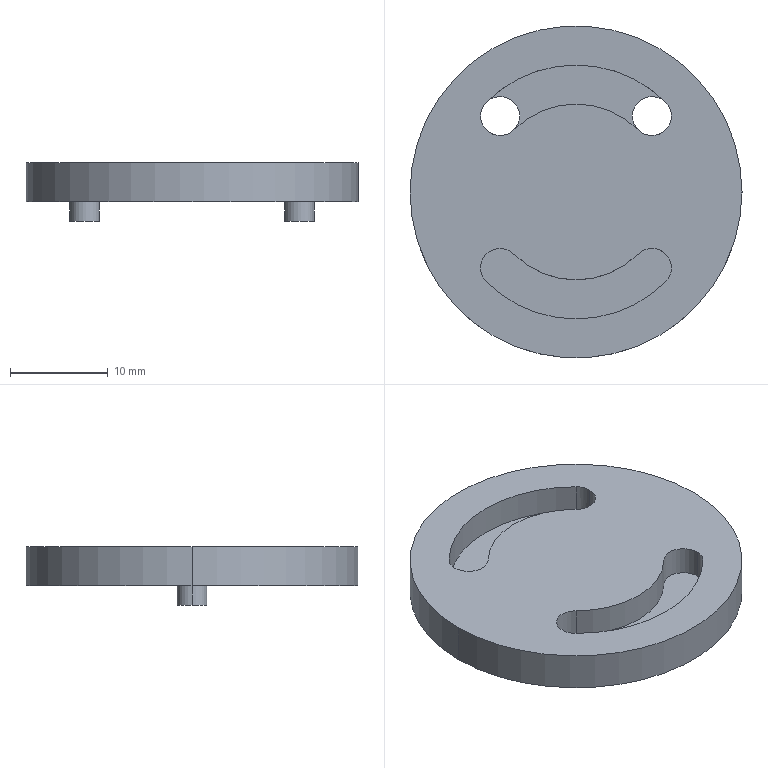Part | SolidWorks | features ICE 4, Extrusion 1 | 1 solid | 23 faces | box 34 x 34 x 6 mm | volume 3145 mm3 | cylinder 17 | plane 6 | commonest cylinder face diameters 4 x7 3 x4 18 x2 26 x2 34 x2
STEP:
#1=CARTESIAN_POINT('',(9.5,0.,-2.));
#2=VERTEX_POINT('',#1);
#3=CARTESIAN_POINT('',(12.5,0.,-2.));
#4=VERTEX_POINT('',#3);
#5=CARTESIAN_POINT('',(11.,0.,-2.));
#6=DIRECTION('',(0.,0.,-1.));
#7=DIRECTION('',(1.,0.,0.));
#8=AXIS2_PLACEMENT_3D('',#5,#6,#7);
#9=CIRCLE('',#8,1.5);
#10=EDGE_CURVE('',#2,#4,#9,.T.);
#11=ORIENTED_EDGE('',*,*,#10,.F.);
#12=CARTESIAN_POINT('',(9.5,0.,0.));
#13=VERTEX_POINT('',#12);
#14=CARTESIAN_POINT('',(9.5,0.,-2.));
#15=DIRECTION('',(0.,0.,1.));
#16=VECTOR('',#15,1000.);
#17=LINE('',#14,#16);
#18=EDGE_CURVE('',#2,#13,#17,.T.);
#19=ORIENTED_EDGE('',*,*,#18,.T.);
#20=CARTESIAN_POINT('',(12.5,0.,0.));
#21=VERTEX_POINT('',#20);
#22=CARTESIAN_POINT('',(11.,0.,0.));
#23=DIRECTION('',(0.,0.,-1.));
#24=DIRECTION('',(1.,0.,0.));
#25=AXIS2_PLACEMENT_3D('',#22,#23,#24);
#26=CIRCLE('',#25,1.5);
#27=EDGE_CURVE('',#13,#21,#26,.T.);
#28=ORIENTED_EDGE('',*,*,#27,.T.);
#29=CARTESIAN_POINT('',(12.5,0.,-2.));
#30=DIRECTION('',(0.,0.,1.));
#31=VECTOR('',#30,1000.);
#32=LINE('',#29,#31);
#33=EDGE_CURVE('',#4,#21,#32,.T.);
#34=ORIENTED_EDGE('',*,*,#33,.F.);
#35=EDGE_LOOP('',(#11,#19,#28,#34));
#36=FACE_OUTER_BOUND('',#35,.T.);
#37=CARTESIAN_POINT('',(11.,0.,-2.));
#38=DIRECTION('',(0.,0.,1.));
#39=DIRECTION('',(1.,0.,0.));
#40=AXIS2_PLACEMENT_3D('',#37,#38,#39);
#41=CYLINDRICAL_SURFACE('',#40,1.5);
#42=ADVANCED_FACE('',(#36),#41,.T.);
#43=CARTESIAN_POINT('',(-12.5,0.,-2.));
#44=VERTEX_POINT('',#43);
#45=CARTESIAN_POINT('',(-9.5,0.,-2.));
#46=VERTEX_POINT('',#45);
#47=CARTESIAN_POINT('',(-11.,0.,-2.));
#48=DIRECTION('',(0.,0.,-1.));
#49=DIRECTION('',(-1.,0.,0.));
#50=AXIS2_PLACEMENT_3D('',#47,#48,#49);
#51=CIRCLE('',#50,1.5);
#52=EDGE_CURVE('',#44,#46,#51,.T.);
#53=ORIENTED_EDGE('',*,*,#52,.F.);
#54=CARTESIAN_POINT('',(-12.5,0.,0.));
#55=VERTEX_POINT('',#54);
#56=CARTESIAN_POINT('',(-12.5,0.,-2.));
#57=DIRECTION('',(0.,0.,1.));
#58=VECTOR('',#57,1000.);
#59=LINE('',#56,#58);
#60=EDGE_CURVE('',#44,#55,#59,.T.);
#61=ORIENTED_EDGE('',*,*,#60,.T.);
#62=CARTESIAN_POINT('',(-9.5,0.,0.));
#63=VERTEX_POINT('',#62);
#64=CARTESIAN_POINT('',(-11.,0.,0.));
#65=DIRECTION('',(0.,0.,-1.));
#66=DIRECTION('',(1.,0.,0.));
#67=AXIS2_PLACEMENT_3D('',#64,#65,#66);
#68=CIRCLE('',#67,1.5);
#69=EDGE_CURVE('',#55,#63,#68,.T.);
#70=ORIENTED_EDGE('',*,*,#69,.T.);
#71=CARTESIAN_POINT('',(-9.5,0.,-2.));
#72=DIRECTION('',(0.,0.,1.));
#73=VECTOR('',#72,1000.);
#74=LINE('',#71,#73);
#75=EDGE_CURVE('',#46,#63,#74,.T.);
#76=ORIENTED_EDGE('',*,*,#75,.F.);
#77=EDGE_LOOP('',(#53,#61,#70,#76));
#78=FACE_OUTER_BOUND('',#77,.T.);
#79=CARTESIAN_POINT('',(-11.,0.,-2.));
#80=DIRECTION('',(0.,0.,1.));
#81=DIRECTION('',(1.,0.,0.));
#82=AXIS2_PLACEMENT_3D('',#79,#80,#81);
#83=CYLINDRICAL_SURFACE('',#82,1.5);
#84=ADVANCED_FACE('',(#78),#83,.T.);
#85=CARTESIAN_POINT('',(9.778,-7.778,1.));
#86=VERTEX_POINT('',#85);
#87=CARTESIAN_POINT('',(6.364,-6.364,1.));
#88=VERTEX_POINT('',#87);
#89=CARTESIAN_POINT('',(7.778,-7.778,1.));
#90=DIRECTION('',(0.,0.,1.));
#91=DIRECTION('',(1.,0.,0.));
#92=AXIS2_PLACEMENT_3D('',#89,#90,#91);
#93=CIRCLE('',#92,2.);
#94=EDGE_CURVE('',#86,#88,#93,.T.);
#95=ORIENTED_EDGE('',*,*,#94,.F.);
#96=CARTESIAN_POINT('',(9.778,-7.778,4.));
#97=VERTEX_POINT('',#96);
#98=CARTESIAN_POINT('',(9.778,-7.778,1.));
#99=DIRECTION('',(0.,0.,1.));
#100=VECTOR('',#99,1000.);
#101=LINE('',#98,#100);
#102=EDGE_CURVE('',#86,#97,#101,.T.);
#103=ORIENTED_EDGE('',*,*,#102,.T.);
#104=CARTESIAN_POINT('',(6.364,-6.364,4.));
#105=VERTEX_POINT('',#104);
#106=CARTESIAN_POINT('',(7.778,-7.778,4.));
#107=DIRECTION('',(0.,0.,1.));
#108=DIRECTION('',(1.,0.,0.));
#109=AXIS2_PLACEMENT_3D('',#106,#107,#108);
#110=CIRCLE('',#109,2.);
#111=EDGE_CURVE('',#97,#105,#110,.T.);
#112=ORIENTED_EDGE('',*,*,#111,.T.);
#113=CARTESIAN_POINT('',(6.364,-6.364,1.));
#114=DIRECTION('',(0.,0.,1.));
#115=VECTOR('',#114,1000.);
#116=LINE('',#113,#115);
#117=EDGE_CURVE('',#88,#105,#116,.T.);
#118=ORIENTED_EDGE('',*,*,#117,.F.);
#119=EDGE_LOOP('',(#95,#103,#112,#118));
#120=FACE_OUTER_BOUND('',#119,.T.);
#121=CARTESIAN_POINT('',(7.778,-7.778,1.));
#122=DIRECTION('',(0.,0.,1.));
#123=DIRECTION('',(1.,0.,0.));
#124=AXIS2_PLACEMENT_3D('',#121,#122,#123);
#125=CYLINDRICAL_SURFACE('',#124,2.);
#126=ADVANCED_FACE('',(#120),#125,.F.);
#127=CARTESIAN_POINT('',(-9.778,7.778,0.));
#128=VERTEX_POINT('',#127);
#129=CARTESIAN_POINT('',(-5.778,7.778,0.));
#130=VERTEX_POINT('',#129);
#131=CARTESIAN_POINT('',(-7.778,7.778,0.));
#132=DIRECTION('',(0.,0.,1.));
#133=DIRECTION('',(1.,0.,0.));
#134=AXIS2_PLACEMENT_3D('',#131,#132,#133);
#135=CIRCLE('',#134,2.);
#136=EDGE_CURVE('',#128,#130,#135,.T.);
#137=ORIENTED_EDGE('',*,*,#136,.F.);
#138=CARTESIAN_POINT('',(-9.778,7.778,4.));
#139=VERTEX_POINT('',#138);
#140=CARTESIAN_POINT('',(-9.778,7.778,1.));
#141=DIRECTION('',(0.,0.,1.));
#142=VECTOR('',#141,1000.);
#143=LINE('',#140,#142);
#144=EDGE_CURVE('',#128,#139,#143,.T.);
#145=ORIENTED_EDGE('',*,*,#144,.T.);
#146=CARTESIAN_POINT('',(-6.364,6.364,4.));
#147=VERTEX_POINT('',#146);
#148=CARTESIAN_POINT('',(-7.778,7.778,4.));
#149=DIRECTION('',(0.,0.,1.));
#150=DIRECTION('',(1.,0.,0.));
#151=AXIS2_PLACEMENT_3D('',#148,#149,#150);
#152=CIRCLE('',#151,2.);
#153=EDGE_CURVE('',#139,#147,#152,.T.);
#154=ORIENTED_EDGE('',*,*,#153,.T.);
#155=CARTESIAN_POINT('',(-6.364,6.364,1.));
#156=VERTEX_POINT('',#155);
#157=CARTESIAN_POINT('',(-6.364,6.364,1.));
#158=DIRECTION('',(0.,0.,1.));
#159=VECTOR('',#158,1000.);
#160=LINE('',#157,#159);
#161=EDGE_CURVE('',#156,#147,#160,.T.);
#162=ORIENTED_EDGE('',*,*,#161,.F.);
#163=CARTESIAN_POINT('',(-5.778,7.778,1.));
#164=VERTEX_POINT('',#163);
#165=CARTESIAN_POINT('',(-7.778,7.778,1.));
#166=DIRECTION('',(0.,0.,1.));
#167=DIRECTION('',(1.,0.,0.));
#168=AXIS2_PLACEMENT_3D('',#165,#166,#167);
#169=CIRCLE('',#168,2.);
#170=EDGE_CURVE('',#156,#164,#169,.T.);
#171=ORIENTED_EDGE('',*,*,#170,.T.);
#172=CARTESIAN_POINT('',(-5.778,7.778,1.));
#173=DIRECTION('',(0.,0.,1.));
#174=VECTOR('',#173,1000.);
#175=LINE('',#172,#174);
#176=EDGE_CURVE('',#130,#164,#175,.T.);
#177=ORIENTED_EDGE('',*,*,#176,.F.);
#178=EDGE_LOOP('',(#137,#145,#154,#162,#171,#177));
#179=FACE_OUTER_BOUND('',#178,.T.);
#180=CARTESIAN_POINT('',(-7.778,7.778,1.));
#181=DIRECTION('',(0.,0.,1.));
#182=DIRECTION('',(1.,0.,0.));
#183=AXIS2_PLACEMENT_3D('',#180,#181,#182);
#184=CYLINDRICAL_SURFACE('',#183,2.);
#185=ADVANCED_FACE('',(#179),#184,.F.);
#186=CARTESIAN_POINT('',(5.778,7.778,0.));
#187=VERTEX_POINT('',#186);
#188=CARTESIAN_POINT('',(9.778,7.778,0.));
#189=VERTEX_POINT('',#188);
#190=CARTESIAN_POINT('',(7.778,7.778,0.));
#191=DIRECTION('',(0.,0.,1.));
#192=DIRECTION('',(1.,0.,0.));
#193=AXIS2_PLACEMENT_3D('',#190,#191,#192);
#194=CIRCLE('',#193,2.);
#195=EDGE_CURVE('',#187,#189,#194,.T.);
#196=ORIENTED_EDGE('',*,*,#195,.F.);
#197=CARTESIAN_POINT('',(5.778,7.778,1.));
#198=VERTEX_POINT('',#197);
#199=CARTESIAN_POINT('',(5.778,7.778,1.));
#200=DIRECTION('',(0.,0.,1.));
#201=VECTOR('',#200,1000.);
#202=LINE('',#199,#201);
#203=EDGE_CURVE('',#187,#198,#202,.T.);
#204=ORIENTED_EDGE('',*,*,#203,.T.);
#205=CARTESIAN_POINT('',(6.364,6.364,1.));
#206=VERTEX_POINT('',#205);
#207=CARTESIAN_POINT('',(7.778,7.778,1.));
#208=DIRECTION('',(0.,0.,1.));
#209=DIRECTION('',(1.,0.,0.));
#210=AXIS2_PLACEMENT_3D('',#207,#208,#209);
#211=CIRCLE('',#210,2.);
#212=EDGE_CURVE('',#198,#206,#211,.T.);
#213=ORIENTED_EDGE('',*,*,#212,.T.);
#214=CARTESIAN_POINT('',(6.364,6.364,4.));
#215=VERTEX_POINT('',#214);
#216=CARTESIAN_POINT('',(6.364,6.364,1.));
#217=DIRECTION('',(0.,0.,1.));
#218=VECTOR('',#217,1000.);
#219=LINE('',#216,#218);
#220=EDGE_CURVE('',#206,#215,#219,.T.);
#221=ORIENTED_EDGE('',*,*,#220,.T.);
#222=CARTESIAN_POINT('',(9.778,7.778,4.));
#223=VERTEX_POINT('',#222);
#224=CARTESIAN_POINT('',(7.778,7.778,4.));
#225=DIRECTION('',(0.,0.,1.));
#226=DIRECTION('',(1.,0.,0.));
#227=AXIS2_PLACEMENT_3D('',#224,#225,#226);
#228=CIRCLE('',#227,2.);
#229=EDGE_CURVE('',#215,#223,#228,.T.);
#230=ORIENTED_EDGE('',*,*,#229,.T.);
#231=CARTESIAN_POINT('',(9.778,7.778,1.));
#232=DIRECTION('',(0.,0.,1.));
#233=VECTOR('',#232,1000.);
#234=LINE('',#231,#233);
#235=EDGE_CURVE('',#189,#223,#234,.T.);
#236=ORIENTED_EDGE('',*,*,#235,.F.);
#237=EDGE_LOOP('',(#196,#204,#213,#221,#230,#236));
#238=FACE_OUTER_BOUND('',#237,.T.);
#239=CARTESIAN_POINT('',(7.778,7.778,1.));
#240=DIRECTION('',(0.,0.,1.));
#241=DIRECTION('',(1.,0.,0.));
#242=AXIS2_PLACEMENT_3D('',#239,#240,#241);
#243=CYLINDRICAL_SURFACE('',#242,2.);
#244=ADVANCED_FACE('',(#238),#243,.F.);
#245=CARTESIAN_POINT('',(17.,0.,4.));
#246=VERTEX_POINT('',#245);
#247=CARTESIAN_POINT('',(-17.,0.,4.));
#248=VERTEX_POINT('',#247);
#249=CARTESIAN_POINT('',(0.,0.,4.));
#250=DIRECTION('',(0.,0.,1.));
#251=DIRECTION('',(1.,0.,0.));
#252=AXIS2_PLACEMENT_3D('',#249,#250,#251);
#253=CIRCLE('',#252,17.);
#254=EDGE_CURVE('',#246,#248,#253,.T.);
#255=ORIENTED_EDGE('',*,*,#254,.F.);
#256=CARTESIAN_POINT('',(17.,0.,0.));
#257=VERTEX_POINT('',#256);
#258=CARTESIAN_POINT('',(17.,0.,4.));
#259=DIRECTION('',(0.,0.,-1.));
#260=VECTOR('',#259,1000.);
#261=LINE('',#258,#260);
#262=EDGE_CURVE('',#246,#257,#261,.T.);
#263=ORIENTED_EDGE('',*,*,#262,.T.);
#264=CARTESIAN_POINT('',(-17.,0.,0.));
#265=VERTEX_POINT('',#264);
#266=CARTESIAN_POINT('',(0.,0.,0.));
#267=DIRECTION('',(0.,0.,1.));
#268=DIRECTION('',(1.,0.,0.));
#269=AXIS2_PLACEMENT_3D('',#266,#267,#268);
#270=CIRCLE('',#269,17.);
#271=EDGE_CURVE('',#257,#265,#270,.T.);
#272=ORIENTED_EDGE('',*,*,#271,.T.);
#273=CARTESIAN_POINT('',(-17.,0.,4.));
#274=DIRECTION('',(0.,0.,-1.));
#275=VECTOR('',#274,1000.);
#276=LINE('',#273,#275);
#277=EDGE_CURVE('',#248,#265,#276,.T.);
#278=ORIENTED_EDGE('',*,*,#277,.F.);
#279=EDGE_LOOP('',(#255,#263,#272,#278));
#280=FACE_OUTER_BOUND('',#279,.T.);
#281=CARTESIAN_POINT('',(0.,0.,4.));
#282=DIRECTION('',(0.,0.,-1.));
#283=DIRECTION('',(-1.,0.,0.));
#284=AXIS2_PLACEMENT_3D('',#281,#282,#283);
#285=CYLINDRICAL_SURFACE('',#284,17.);
#286=ADVANCED_FACE('',(#280),#285,.T.);
#287=ORIENTED_EDGE('',*,*,#262,.F.);
#288=CARTESIAN_POINT('',(0.,0.,4.));
#289=DIRECTION('',(0.,0.,1.));
#290=DIRECTION('',(1.,0.,0.));
#291=AXIS2_PLACEMENT_3D('',#288,#289,#290);
#292=CIRCLE('',#291,17.);
#293=EDGE_CURVE('',#248,#246,#292,.T.);
#294=ORIENTED_EDGE('',*,*,#293,.F.);
#295=ORIENTED_EDGE('',*,*,#277,.T.);
#296=CARTESIAN_POINT('',(0.,0.,0.));
#297=DIRECTION('',(0.,0.,1.));
#298=DIRECTION('',(1.,0.,0.));
#299=AXIS2_PLACEMENT_3D('',#296,#297,#298);
#300=CIRCLE('',#299,17.);
#301=EDGE_CURVE('',#265,#257,#300,.T.);
#302=ORIENTED_EDGE('',*,*,#301,.T.);
#303=EDGE_LOOP('',(#287,#294,#295,#302));
#304=FACE_OUTER_BOUND('',#303,.T.);
#305=CARTESIAN_POINT('',(0.,0.,4.));
#306=DIRECTION('',(0.,0.,-1.));
#307=DIRECTION('',(-1.,0.,0.));
#308=AXIS2_PLACEMENT_3D('',#305,#306,#307);
#309=CYLINDRICAL_SURFACE('',#308,17.);
#310=ADVANCED_FACE('',(#304),#309,.T.);
#311=CARTESIAN_POINT('',(-6.364,-6.364,4.));
#312=VERTEX_POINT('',#311);
#313=CARTESIAN_POINT('',(-9.192,-9.192,4.));
#314=VERTEX_POINT('',#313);
#315=CARTESIAN_POINT('',(-7.778,-7.778,4.));
#316=DIRECTION('',(0.,0.,1.));
#317=DIRECTION('',(1.,0.,0.));
#318=AXIS2_PLACEMENT_3D('',#315,#316,#317);
#319=CIRCLE('',#318,2.);
#320=EDGE_CURVE('',#312,#314,#319,.T.);
#321=ORIENTED_EDGE('',*,*,#320,.F.);
#322=CARTESIAN_POINT('',(0.,0.,4.));
#323=DIRECTION('',(0.,0.,-1.));
#324=DIRECTION('',(1.,0.,0.));
#325=AXIS2_PLACEMENT_3D('',#322,#323,#324);
#326=CIRCLE('',#325,9.);
#327=EDGE_CURVE('',#105,#312,#326,.T.);
#328=ORIENTED_EDGE('',*,*,#327,.F.);
#329=ORIENTED_EDGE('',*,*,#111,.F.);
#330=CARTESIAN_POINT('',(9.192,-9.192,4.));
#331=VERTEX_POINT('',#330);
#332=CARTESIAN_POINT('',(7.778,-7.778,4.));
#333=DIRECTION('',(0.,0.,1.));
#334=DIRECTION('',(1.,0.,0.));
#335=AXIS2_PLACEMENT_3D('',#332,#333,#334);
#336=CIRCLE('',#335,2.);
#337=EDGE_CURVE('',#331,#97,#336,.T.);
#338=ORIENTED_EDGE('',*,*,#337,.F.);
#339=CARTESIAN_POINT('',(0.,0.,4.));
#340=DIRECTION('',(0.,0.,1.));
#341=DIRECTION('',(1.,0.,0.));
#342=AXIS2_PLACEMENT_3D('',#339,#340,#341);
#343=CIRCLE('',#342,13.);
#344=EDGE_CURVE('',#314,#331,#343,.T.);
#345=ORIENTED_EDGE('',*,*,#344,.F.);
#346=EDGE_LOOP('',(#321,#328,#329,#338,#345));
#347=FACE_BOUND('',#346,.T.);
#348=ORIENTED_EDGE('',*,*,#229,.F.);
#349=CARTESIAN_POINT('',(0.,0.,4.));
#350=DIRECTION('',(0.,0.,-1.));
#351=DIRECTION('',(1.,0.,0.));
#352=AXIS2_PLACEMENT_3D('',#349,#350,#351);
#353=CIRCLE('',#352,9.);
#354=EDGE_CURVE('',#147,#215,#353,.T.);
#355=ORIENTED_EDGE('',*,*,#354,.F.);
#356=ORIENTED_EDGE('',*,*,#153,.F.);
#357=CARTESIAN_POINT('',(-9.192,9.192,4.));
#358=VERTEX_POINT('',#357);
#359=CARTESIAN_POINT('',(-7.778,7.778,4.));
#360=DIRECTION('',(0.,0.,1.));
#361=DIRECTION('',(1.,0.,0.));
#362=AXIS2_PLACEMENT_3D('',#359,#360,#361);
#363=CIRCLE('',#362,2.);
#364=EDGE_CURVE('',#358,#139,#363,.T.);
#365=ORIENTED_EDGE('',*,*,#364,.F.);
#366=CARTESIAN_POINT('',(9.192,9.192,4.));
#367=VERTEX_POINT('',#366);
#368=CARTESIAN_POINT('',(0.,0.,4.));
#369=DIRECTION('',(0.,0.,1.));
#370=DIRECTION('',(1.,0.,0.));
#371=AXIS2_PLACEMENT_3D('',#368,#369,#370);
#372=CIRCLE('',#371,13.);
#373=EDGE_CURVE('',#367,#358,#372,.T.);
#374=ORIENTED_EDGE('',*,*,#373,.F.);
#375=CARTESIAN_POINT('',(7.778,7.778,4.));
#376=DIRECTION('',(0.,0.,1.));
#377=DIRECTION('',(1.,0.,0.));
#378=AXIS2_PLACEMENT_3D('',#375,#376,#377);
#379=CIRCLE('',#378,2.);
#380=EDGE_CURVE('',#223,#367,#379,.T.);
#381=ORIENTED_EDGE('',*,*,#380,.F.);
#382=EDGE_LOOP('',(#348,#355,#356,#365,#374,#381));
#383=FACE_BOUND('',#382,.T.);
#384=ORIENTED_EDGE('',*,*,#293,.T.);
#385=ORIENTED_EDGE('',*,*,#254,.T.);
#386=EDGE_LOOP('',(#384,#385));
#387=FACE_OUTER_BOUND('',#386,.T.);
#388=CARTESIAN_POINT('',(0.,0.,4.));
#389=DIRECTION('',(0.,0.,1.));
#390=DIRECTION('',(1.,0.,0.));
#391=AXIS2_PLACEMENT_3D('',#388,#389,#390);
#392=PLANE('',#391);
#393=ADVANCED_FACE('',(#347,#383,#387),#392,.T.);
#394=CARTESIAN_POINT('',(11.,0.,0.));
#395=DIRECTION('',(0.,0.,-1.));
#396=DIRECTION('',(1.,0.,0.));
#397=AXIS2_PLACEMENT_3D('',#394,#395,#396);
#398=CIRCLE('',#397,1.5);
#399=EDGE_CURVE('',#21,#13,#398,.T.);
#400=ORIENTED_EDGE('',*,*,#399,.F.);
#401=ORIENTED_EDGE('',*,*,#27,.F.);
#402=EDGE_LOOP('',(#400,#401));
#403=FACE_BOUND('',#402,.T.);
#404=CARTESIAN_POINT('',(-11.,0.,0.));
#405=DIRECTION('',(0.,0.,-1.));
#406=DIRECTION('',(1.,0.,0.));
#407=AXIS2_PLACEMENT_3D('',#404,#405,#406);
#408=CIRCLE('',#407,1.5);
#409=EDGE_CURVE('',#63,#55,#408,.T.);
#410=ORIENTED_EDGE('',*,*,#409,.F.);
#411=ORIENTED_EDGE('',*,*,#69,.F.);
#412=EDGE_LOOP('',(#410,#411));
#413=FACE_BOUND('',#412,.T.);
#414=CARTESIAN_POINT('',(7.778,7.778,0.));
#415=DIRECTION('',(0.,0.,1.));
#416=DIRECTION('',(1.,0.,0.));
#417=AXIS2_PLACEMENT_3D('',#414,#415,#416);
#418=CIRCLE('',#417,2.);
#419=EDGE_CURVE('',#189,#187,#418,.T.);
#420=ORIENTED_EDGE('',*,*,#419,.T.);
#421=ORIENTED_EDGE('',*,*,#195,.T.);
#422=EDGE_LOOP('',(#420,#421));
#423=FACE_BOUND('',#422,.T.);
#424=CARTESIAN_POINT('',(-7.778,7.778,0.));
#425=DIRECTION('',(0.,0.,1.));
#426=DIRECTION('',(1.,0.,0.));
#427=AXIS2_PLACEMENT_3D('',#424,#425,#426);
#428=CIRCLE('',#427,2.);
#429=EDGE_CURVE('',#130,#128,#428,.T.);
#430=ORIENTED_EDGE('',*,*,#429,.T.);
#431=ORIENTED_EDGE('',*,*,#136,.T.);
#432=EDGE_LOOP('',(#430,#431));
#433=FACE_BOUND('',#432,.T.);
#434=ORIENTED_EDGE('',*,*,#301,.F.);
#435=ORIENTED_EDGE('',*,*,#271,.F.);
#436=EDGE_LOOP('',(#434,#435));
#437=FACE_OUTER_BOUND('',#436,.T.);
#438=CARTESIAN_POINT('',(0.,0.,0.));
#439=DIRECTION('',(0.,0.,1.));
#440=DIRECTION('',(1.,0.,0.));
#441=AXIS2_PLACEMENT_3D('',#438,#439,#440);
#442=PLANE('',#441);
#443=ADVANCED_FACE('',(#403,#413,#423,#433,#437),#442,.F.);
#444=ORIENTED_EDGE('',*,*,#203,.F.);
#445=ORIENTED_EDGE('',*,*,#419,.F.);
#446=ORIENTED_EDGE('',*,*,#235,.T.);
#447=ORIENTED_EDGE('',*,*,#380,.T.);
#448=CARTESIAN_POINT('',(9.192,9.192,1.));
#449=VERTEX_POINT('',#448);
#450=CARTESIAN_POINT('',(9.192,9.192,1.));
#451=DIRECTION('',(0.,0.,1.));
#452=VECTOR('',#451,1000.);
#453=LINE('',#450,#452);
#454=EDGE_CURVE('',#449,#367,#453,.T.);
#455=ORIENTED_EDGE('',*,*,#454,.F.);
#456=CARTESIAN_POINT('',(7.778,7.778,1.));
#457=DIRECTION('',(0.,0.,1.));
#458=DIRECTION('',(1.,0.,0.));
#459=AXIS2_PLACEMENT_3D('',#456,#457,#458);
#460=CIRCLE('',#459,2.);
#461=EDGE_CURVE('',#449,#198,#460,.T.);
#462=ORIENTED_EDGE('',*,*,#461,.T.);
#463=EDGE_LOOP('',(#444,#445,#446,#447,#455,#462));
#464=FACE_OUTER_BOUND('',#463,.T.);
#465=CARTESIAN_POINT('',(7.778,7.778,1.));
#466=DIRECTION('',(0.,0.,1.));
#467=DIRECTION('',(1.,0.,0.));
#468=AXIS2_PLACEMENT_3D('',#465,#466,#467);
#469=CYLINDRICAL_SURFACE('',#468,2.);
#470=ADVANCED_FACE('',(#464),#469,.F.);
#471=ORIENTED_EDGE('',*,*,#354,.T.);
#472=ORIENTED_EDGE('',*,*,#220,.F.);
#473=CARTESIAN_POINT('',(0.,0.,1.));
#474=DIRECTION('',(0.,0.,-1.));
#475=DIRECTION('',(1.,0.,0.));
#476=AXIS2_PLACEMENT_3D('',#473,#474,#475);
#477=CIRCLE('',#476,9.);
#478=EDGE_CURVE('',#156,#206,#477,.T.);
#479=ORIENTED_EDGE('',*,*,#478,.F.);
#480=ORIENTED_EDGE('',*,*,#161,.T.);
#481=EDGE_LOOP('',(#471,#472,#479,#480));
#482=FACE_OUTER_BOUND('',#481,.T.);
#483=CARTESIAN_POINT('',(0.,0.,1.));
#484=DIRECTION('',(0.,0.,1.));
#485=DIRECTION('',(1.,0.,0.));
#486=AXIS2_PLACEMENT_3D('',#483,#484,#485);
#487=CYLINDRICAL_SURFACE('',#486,9.);
#488=ADVANCED_FACE('',(#482),#487,.T.);
#489=ORIENTED_EDGE('',*,*,#144,.F.);
#490=ORIENTED_EDGE('',*,*,#429,.F.);
#491=ORIENTED_EDGE('',*,*,#176,.T.);
#492=CARTESIAN_POINT('',(-9.192,9.192,1.));
#493=VERTEX_POINT('',#492);
#494=CARTESIAN_POINT('',(-7.778,7.778,1.));
#495=DIRECTION('',(0.,0.,1.));
#496=DIRECTION('',(1.,0.,0.));
#497=AXIS2_PLACEMENT_3D('',#494,#495,#496);
#498=CIRCLE('',#497,2.);
#499=EDGE_CURVE('',#164,#493,#498,.T.);
#500=ORIENTED_EDGE('',*,*,#499,.T.);
#501=CARTESIAN_POINT('',(-9.192,9.192,1.));
#502=DIRECTION('',(0.,0.,1.));
#503=VECTOR('',#502,1000.);
#504=LINE('',#501,#503);
#505=EDGE_CURVE('',#493,#358,#504,.T.);
#506=ORIENTED_EDGE('',*,*,#505,.T.);
#507=ORIENTED_EDGE('',*,*,#364,.T.);
#508=EDGE_LOOP('',(#489,#490,#491,#500,#506,#507));
#509=FACE_OUTER_BOUND('',#508,.T.);
#510=CARTESIAN_POINT('',(-7.778,7.778,1.));
#511=DIRECTION('',(0.,0.,1.));
#512=DIRECTION('',(1.,0.,0.));
#513=AXIS2_PLACEMENT_3D('',#510,#511,#512);
#514=CYLINDRICAL_SURFACE('',#513,2.);
#515=ADVANCED_FACE('',(#509),#514,.F.);
#516=ORIENTED_EDGE('',*,*,#373,.T.);
#517=ORIENTED_EDGE('',*,*,#505,.F.);
#518=CARTESIAN_POINT('',(0.,0.,1.));
#519=DIRECTION('',(0.,0.,1.));
#520=DIRECTION('',(1.,0.,0.));
#521=AXIS2_PLACEMENT_3D('',#518,#519,#520);
#522=CIRCLE('',#521,13.);
#523=EDGE_CURVE('',#449,#493,#522,.T.);
#524=ORIENTED_EDGE('',*,*,#523,.F.);
#525=ORIENTED_EDGE('',*,*,#454,.T.);
#526=EDGE_LOOP('',(#516,#517,#524,#525));
#527=FACE_OUTER_BOUND('',#526,.T.);
#528=CARTESIAN_POINT('',(0.,0.,1.));
#529=DIRECTION('',(0.,0.,1.));
#530=DIRECTION('',(1.,0.,0.));
#531=AXIS2_PLACEMENT_3D('',#528,#529,#530);
#532=CYLINDRICAL_SURFACE('',#531,13.);
#533=ADVANCED_FACE('',(#527),#532,.F.);
#534=ORIENTED_EDGE('',*,*,#461,.F.);
#535=ORIENTED_EDGE('',*,*,#523,.T.);
#536=ORIENTED_EDGE('',*,*,#499,.F.);
#537=ORIENTED_EDGE('',*,*,#170,.F.);
#538=ORIENTED_EDGE('',*,*,#478,.T.);
#539=ORIENTED_EDGE('',*,*,#212,.F.);
#540=EDGE_LOOP('',(#534,#535,#536,#537,#538,#539));
#541=FACE_OUTER_BOUND('',#540,.T.);
#542=CARTESIAN_POINT('',(3.889,3.889,1.));
#543=DIRECTION('',(0.,0.,1.));
#544=DIRECTION('',(1.,0.,0.));
#545=AXIS2_PLACEMENT_3D('',#542,#543,#544);
#546=PLANE('',#545);
#547=ADVANCED_FACE('',(#541),#546,.T.);
#548=ORIENTED_EDGE('',*,*,#320,.T.);
#549=CARTESIAN_POINT('',(-9.192,-9.192,1.));
#550=VERTEX_POINT('',#549);
#551=CARTESIAN_POINT('',(-9.192,-9.192,1.));
#552=DIRECTION('',(0.,0.,1.));
#553=VECTOR('',#552,1000.);
#554=LINE('',#551,#553);
#555=EDGE_CURVE('',#550,#314,#554,.T.);
#556=ORIENTED_EDGE('',*,*,#555,.F.);
#557=CARTESIAN_POINT('',(-6.364,-6.364,1.));
#558=VERTEX_POINT('',#557);
#559=CARTESIAN_POINT('',(-7.778,-7.778,1.));
#560=DIRECTION('',(0.,0.,1.));
#561=DIRECTION('',(1.,0.,0.));
#562=AXIS2_PLACEMENT_3D('',#559,#560,#561);
#563=CIRCLE('',#562,2.);
#564=EDGE_CURVE('',#558,#550,#563,.T.);
#565=ORIENTED_EDGE('',*,*,#564,.F.);
#566=CARTESIAN_POINT('',(-6.364,-6.364,1.));
#567=DIRECTION('',(0.,0.,1.));
#568=VECTOR('',#567,1000.);
#569=LINE('',#566,#568);
#570=EDGE_CURVE('',#558,#312,#569,.T.);
#571=ORIENTED_EDGE('',*,*,#570,.T.);
#572=EDGE_LOOP('',(#548,#556,#565,#571));
#573=FACE_OUTER_BOUND('',#572,.T.);
#574=CARTESIAN_POINT('',(-7.778,-7.778,1.));
#575=DIRECTION('',(0.,0.,1.));
#576=DIRECTION('',(1.,0.,0.));
#577=AXIS2_PLACEMENT_3D('',#574,#575,#576);
#578=CYLINDRICAL_SURFACE('',#577,2.);
#579=ADVANCED_FACE('',(#573),#578,.F.);
#580=ORIENTED_EDGE('',*,*,#327,.T.);
#581=ORIENTED_EDGE('',*,*,#570,.F.);
#582=CARTESIAN_POINT('',(0.,0.,1.));
#583=DIRECTION('',(0.,0.,-1.));
#584=DIRECTION('',(1.,0.,0.));
#585=AXIS2_PLACEMENT_3D('',#582,#583,#584);
#586=CIRCLE('',#585,9.);
#587=EDGE_CURVE('',#88,#558,#586,.T.);
#588=ORIENTED_EDGE('',*,*,#587,.F.);
#589=ORIENTED_EDGE('',*,*,#117,.T.);
#590=EDGE_LOOP('',(#580,#581,#588,#589));
#591=FACE_OUTER_BOUND('',#590,.T.);
#592=CARTESIAN_POINT('',(0.,0.,1.));
#593=DIRECTION('',(0.,0.,1.));
#594=DIRECTION('',(1.,0.,0.));
#595=AXIS2_PLACEMENT_3D('',#592,#593,#594);
#596=CYLINDRICAL_SURFACE('',#595,9.);
#597=ADVANCED_FACE('',(#591),#596,.T.);
#598=ORIENTED_EDGE('',*,*,#102,.F.);
#599=CARTESIAN_POINT('',(9.192,-9.192,1.));
#600=VERTEX_POINT('',#599);
#601=CARTESIAN_POINT('',(7.778,-7.778,1.));
#602=DIRECTION('',(0.,0.,1.));
#603=DIRECTION('',(1.,0.,0.));
#604=AXIS2_PLACEMENT_3D('',#601,#602,#603);
#605=CIRCLE('',#604,2.);
#606=EDGE_CURVE('',#600,#86,#605,.T.);
#607=ORIENTED_EDGE('',*,*,#606,.F.);
#608=CARTESIAN_POINT('',(9.192,-9.192,1.));
#609=DIRECTION('',(0.,0.,1.));
#610=VECTOR('',#609,1000.);
#611=LINE('',#608,#610);
#612=EDGE_CURVE('',#600,#331,#611,.T.);
#613=ORIENTED_EDGE('',*,*,#612,.T.);
#614=ORIENTED_EDGE('',*,*,#337,.T.);
#615=EDGE_LOOP('',(#598,#607,#613,#614));
#616=FACE_OUTER_BOUND('',#615,.T.);
#617=CARTESIAN_POINT('',(7.778,-7.778,1.));
#618=DIRECTION('',(0.,0.,1.));
#619=DIRECTION('',(1.,0.,0.));
#620=AXIS2_PLACEMENT_3D('',#617,#618,#619);
#621=CYLINDRICAL_SURFACE('',#620,2.);
#622=ADVANCED_FACE('',(#616),#621,.F.);
#623=ORIENTED_EDGE('',*,*,#344,.T.);
#624=ORIENTED_EDGE('',*,*,#612,.F.);
#625=CARTESIAN_POINT('',(0.,0.,1.));
#626=DIRECTION('',(0.,0.,1.));
#627=DIRECTION('',(1.,0.,0.));
#628=AXIS2_PLACEMENT_3D('',#625,#626,#627);
#629=CIRCLE('',#628,13.);
#630=EDGE_CURVE('',#550,#600,#629,.T.);
#631=ORIENTED_EDGE('',*,*,#630,.F.);
#632=ORIENTED_EDGE('',*,*,#555,.T.);
#633=EDGE_LOOP('',(#623,#624,#631,#632));
#634=FACE_OUTER_BOUND('',#633,.T.);
#635=CARTESIAN_POINT('',(0.,0.,1.));
#636=DIRECTION('',(0.,0.,1.));
#637=DIRECTION('',(1.,0.,0.));
#638=AXIS2_PLACEMENT_3D('',#635,#636,#637);
#639=CYLINDRICAL_SURFACE('',#638,13.);
#640=ADVANCED_FACE('',(#634),#639,.F.);
#641=ORIENTED_EDGE('',*,*,#564,.T.);
#642=ORIENTED_EDGE('',*,*,#630,.T.);
#643=ORIENTED_EDGE('',*,*,#606,.T.);
#644=ORIENTED_EDGE('',*,*,#94,.T.);
#645=ORIENTED_EDGE('',*,*,#587,.T.);
#646=EDGE_LOOP('',(#641,#642,#643,#644,#645));
#647=FACE_OUTER_BOUND('',#646,.T.);
#648=CARTESIAN_POINT('',(-3.889,-3.889,1.));
#649=DIRECTION('',(0.,0.,1.));
#650=DIRECTION('',(1.,0.,0.));
#651=AXIS2_PLACEMENT_3D('',#648,#649,#650);
#652=PLANE('',#651);
#653=ADVANCED_FACE('',(#647),#652,.T.);
#654=ORIENTED_EDGE('',*,*,#60,.F.);
#655=CARTESIAN_POINT('',(-11.,0.,-2.));
#656=DIRECTION('',(0.,0.,-1.));
#657=DIRECTION('',(-1.,0.,0.));
#658=AXIS2_PLACEMENT_3D('',#655,#656,#657);
#659=CIRCLE('',#658,1.5);
#660=EDGE_CURVE('',#46,#44,#659,.T.);
#661=ORIENTED_EDGE('',*,*,#660,.F.);
#662=ORIENTED_EDGE('',*,*,#75,.T.);
#663=ORIENTED_EDGE('',*,*,#409,.T.);
#664=EDGE_LOOP('',(#654,#661,#662,#663));
#665=FACE_OUTER_BOUND('',#664,.T.);
#666=CARTESIAN_POINT('',(-11.,0.,-2.));
#667=DIRECTION('',(0.,0.,1.));
#668=DIRECTION('',(1.,0.,0.));
#669=AXIS2_PLACEMENT_3D('',#666,#667,#668);
#670=CYLINDRICAL_SURFACE('',#669,1.5);
#671=ADVANCED_FACE('',(#665),#670,.T.);
#672=ORIENTED_EDGE('',*,*,#660,.T.);
#673=ORIENTED_EDGE('',*,*,#52,.T.);
#674=EDGE_LOOP('',(#672,#673));
#675=FACE_OUTER_BOUND('',#674,.T.);
#676=CARTESIAN_POINT('',(-11.,0.,-2.));
#677=DIRECTION('',(0.,0.,-1.));
#678=DIRECTION('',(-1.,0.,0.));
#679=AXIS2_PLACEMENT_3D('',#676,#677,#678);
#680=PLANE('',#679);
#681=ADVANCED_FACE('',(#675),#680,.T.);
#682=ORIENTED_EDGE('',*,*,#18,.F.);
#683=CARTESIAN_POINT('',(11.,0.,-2.));
#684=DIRECTION('',(0.,0.,-1.));
#685=DIRECTION('',(1.,0.,0.));
#686=AXIS2_PLACEMENT_3D('',#683,#684,#685);
#687=CIRCLE('',#686,1.5);
#688=EDGE_CURVE('',#4,#2,#687,.T.);
#689=ORIENTED_EDGE('',*,*,#688,.F.);
#690=ORIENTED_EDGE('',*,*,#33,.T.);
#691=ORIENTED_EDGE('',*,*,#399,.T.);
#692=EDGE_LOOP('',(#682,#689,#690,#691));
#693=FACE_OUTER_BOUND('',#692,.T.);
#694=CARTESIAN_POINT('',(11.,0.,-2.));
#695=DIRECTION('',(0.,0.,1.));
#696=DIRECTION('',(1.,0.,0.));
#697=AXIS2_PLACEMENT_3D('',#694,#695,#696);
#698=CYLINDRICAL_SURFACE('',#697,1.5);
#699=ADVANCED_FACE('',(#693),#698,.T.);
#700=ORIENTED_EDGE('',*,*,#688,.T.);
#701=ORIENTED_EDGE('',*,*,#10,.T.);
#702=EDGE_LOOP('',(#700,#701));
#703=FACE_OUTER_BOUND('',#702,.T.);
#704=CARTESIAN_POINT('',(11.,0.,-2.));
#705=DIRECTION('',(0.,0.,1.));
#706=DIRECTION('',(1.,0.,0.));
#707=AXIS2_PLACEMENT_3D('',#704,#705,#706);
#708=PLANE('',#707);
#709=ADVANCED_FACE('',(#703),#708,.F.);
#710=CLOSED_SHELL('',(#42,#84,#126,#185,#244,#286,#310,#393,#443,#470,#488,#515,#533,#547,#579,#597,#622,#640,#653,#671,#681,#699,#709));
#711=MANIFOLD_SOLID_BREP('',#710);
#712=CARTESIAN_POINT('',(0.,0.,0.));
#713=DIRECTION('',(0.,0.,1.));
#714=DIRECTION('',(1.,0.,0.));
#715=AXIS2_PLACEMENT_3D('',#712,#713,#714);
#716=(LENGTH_UNIT()NAMED_UNIT(*)SI_UNIT(.MILLI.,.METRE.));
#717=UNCERTAINTY_MEASURE_WITH_UNIT(LENGTH_MEASURE(0.00001),#716,'','');
#718=(NAMED_UNIT(*)PLANE_ANGLE_UNIT()SI_UNIT($,.RADIAN.));
#719=(NAMED_UNIT(*)SI_UNIT($,.STERADIAN.)SOLID_ANGLE_UNIT());
#720=(GEOMETRIC_REPRESENTATION_CONTEXT(3)GLOBAL_UNCERTAINTY_ASSIGNED_CONTEXT((#717))GLOBAL_UNIT_ASSIGNED_CONTEXT((#716,#718,#719))REPRESENTATION_CONTEXT('',''));
#721=ADVANCED_BREP_SHAPE_REPRESENTATION('',(#711,#715),#720);